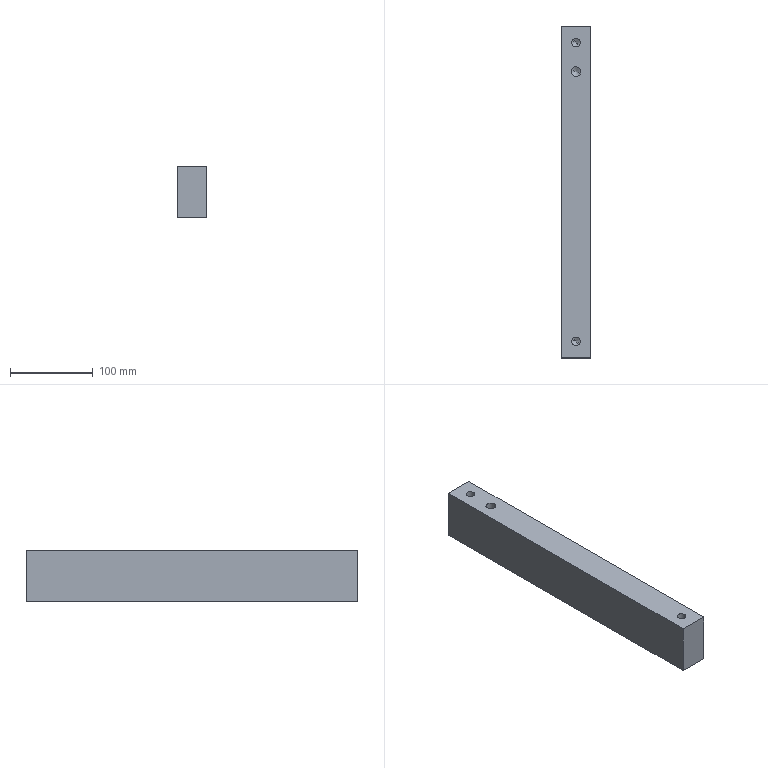Part | CATIA | 1 solid | 38 faces | box 35 x 400 x 61.7 mm | volume 838529 mm3 | cone 16 | cylinder 16 | plane 6 | commonest cylinder face diameters 10.2 x10 12 x6
STEP:
#1=CARTESIAN_POINT('',(-17.5,200.,-275.));
#2=VERTEX_POINT('',#1);
#3=CARTESIAN_POINT('',(-17.5,-200.,-275.));
#4=VERTEX_POINT('',#3);
#5=CARTESIAN_POINT('',(-17.5,0.,-275.));
#6=DIRECTION('',(0.,-1.,0.));
#7=VECTOR('',#6,1.);
#8=LINE('',#5,#7);
#9=EDGE_CURVE('',#2,#4,#8,.T.);
#10=ORIENTED_EDGE('',*,*,#9,.T.);
#11=CARTESIAN_POINT('',(-17.5,-200.,-213.3));
#12=VERTEX_POINT('',#11);
#13=CARTESIAN_POINT('',(-17.5,-200.,-244.15));
#14=DIRECTION('',(0.,0.,-1.));
#15=VECTOR('',#14,1.);
#16=LINE('',#13,#15);
#17=EDGE_CURVE('',#12,#4,#16,.T.);
#18=ORIENTED_EDGE('',*,*,#17,.F.);
#19=CARTESIAN_POINT('',(-17.5,200.,-213.3));
#20=VERTEX_POINT('',#19);
#21=CARTESIAN_POINT('',(-17.5,0.,-213.3));
#22=DIRECTION('',(0.,-1.,0.));
#23=VECTOR('',#22,1.);
#24=LINE('',#21,#23);
#25=EDGE_CURVE('',#20,#12,#24,.T.);
#26=ORIENTED_EDGE('',*,*,#25,.F.);
#27=CARTESIAN_POINT('',(-17.5,200.,-244.15));
#28=DIRECTION('',(0.,0.,-1.));
#29=VECTOR('',#28,1.);
#30=LINE('',#27,#29);
#31=EDGE_CURVE('',#20,#2,#30,.T.);
#32=ORIENTED_EDGE('',*,*,#31,.T.);
#33=EDGE_LOOP('',(#10,#18,#26,#32));
#34=FACE_OUTER_BOUND('',#33,.T.);
#35=CARTESIAN_POINT('',(-17.5,200.,0.));
#36=DIRECTION('',(1.,0.,0.));
#37=DIRECTION('',(0.,-1.,0.));
#38=AXIS2_PLACEMENT_3D('',#35,#36,#37);
#39=PLANE('',#38);
#40=ADVANCED_FACE('',(#34),#39,.F.);
#41=CARTESIAN_POINT('',(17.5,-200.,-275.));
#42=VERTEX_POINT('',#41);
#43=CARTESIAN_POINT('',(0.,-200.,-275.));
#44=DIRECTION('',(-1.,0.,0.));
#45=VECTOR('',#44,1.);
#46=LINE('',#43,#45);
#47=EDGE_CURVE('',#4,#42,#46,.F.);
#48=ORIENTED_EDGE('',*,*,#47,.T.);
#49=CARTESIAN_POINT('',(17.5,-200.,-213.3));
#50=VERTEX_POINT('',#49);
#51=CARTESIAN_POINT('',(17.5,-200.,-244.15));
#52=DIRECTION('',(0.,0.,-1.));
#53=VECTOR('',#52,1.);
#54=LINE('',#51,#53);
#55=EDGE_CURVE('',#50,#42,#54,.T.);
#56=ORIENTED_EDGE('',*,*,#55,.F.);
#57=CARTESIAN_POINT('',(0.,-200.,-213.3));
#58=DIRECTION('',(-1.,0.,0.));
#59=VECTOR('',#58,1.);
#60=LINE('',#57,#59);
#61=EDGE_CURVE('',#12,#50,#60,.F.);
#62=ORIENTED_EDGE('',*,*,#61,.F.);
#63=ORIENTED_EDGE('',*,*,#17,.T.);
#64=EDGE_LOOP('',(#48,#56,#62,#63));
#65=FACE_OUTER_BOUND('',#64,.T.);
#66=CARTESIAN_POINT('',(17.5,-200.,0.));
#67=DIRECTION('',(0.,-1.,0.));
#68=DIRECTION('',(-1.,0.,0.));
#69=AXIS2_PLACEMENT_3D('',#66,#67,#68);
#70=PLANE('',#69);
#71=ADVANCED_FACE('',(#65),#70,.T.);
#72=CARTESIAN_POINT('',(17.5,200.,-275.));
#73=VERTEX_POINT('',#72);
#74=CARTESIAN_POINT('',(17.5,0.,-275.));
#75=DIRECTION('',(0.,1.,0.));
#76=VECTOR('',#75,1.);
#77=LINE('',#74,#76);
#78=EDGE_CURVE('',#42,#73,#77,.T.);
#79=ORIENTED_EDGE('',*,*,#78,.T.);
#80=CARTESIAN_POINT('',(17.5,200.,-213.3));
#81=VERTEX_POINT('',#80);
#82=CARTESIAN_POINT('',(17.5,200.,-244.15));
#83=DIRECTION('',(0.,0.,-1.));
#84=VECTOR('',#83,1.);
#85=LINE('',#82,#84);
#86=EDGE_CURVE('',#81,#73,#85,.T.);
#87=ORIENTED_EDGE('',*,*,#86,.F.);
#88=CARTESIAN_POINT('',(17.5,0.,-213.3));
#89=DIRECTION('',(0.,1.,0.));
#90=VECTOR('',#89,1.);
#91=LINE('',#88,#90);
#92=EDGE_CURVE('',#50,#81,#91,.T.);
#93=ORIENTED_EDGE('',*,*,#92,.F.);
#94=ORIENTED_EDGE('',*,*,#55,.T.);
#95=EDGE_LOOP('',(#79,#87,#93,#94));
#96=FACE_OUTER_BOUND('',#95,.T.);
#97=CARTESIAN_POINT('',(17.5,-200.,0.));
#98=DIRECTION('',(-1.,0.,0.));
#99=DIRECTION('',(0.,1.,0.));
#100=AXIS2_PLACEMENT_3D('',#97,#98,#99);
#101=PLANE('',#100);
#102=ADVANCED_FACE('',(#96),#101,.F.);
#103=CARTESIAN_POINT('',(0.,200.,-275.));
#104=DIRECTION('',(1.,0.,0.));
#105=VECTOR('',#104,1.);
#106=LINE('',#103,#105);
#107=EDGE_CURVE('',#73,#2,#106,.F.);
#108=ORIENTED_EDGE('',*,*,#107,.T.);
#109=ORIENTED_EDGE('',*,*,#31,.F.);
#110=CARTESIAN_POINT('',(0.,200.,-213.3));
#111=DIRECTION('',(1.,0.,0.));
#112=VECTOR('',#111,1.);
#113=LINE('',#110,#112);
#114=EDGE_CURVE('',#81,#20,#113,.F.);
#115=ORIENTED_EDGE('',*,*,#114,.F.);
#116=ORIENTED_EDGE('',*,*,#86,.T.);
#117=EDGE_LOOP('',(#108,#109,#115,#116));
#118=FACE_OUTER_BOUND('',#117,.T.);
#119=CARTESIAN_POINT('',(-17.5,200.,0.));
#120=DIRECTION('',(0.,1.,0.));
#121=DIRECTION('',(1.,0.,0.));
#122=AXIS2_PLACEMENT_3D('',#119,#120,#121);
#123=PLANE('',#122);
#124=ADVANCED_FACE('',(#118),#123,.T.);
#125=ORIENTED_EDGE('',*,*,#107,.F.);
#126=ORIENTED_EDGE('',*,*,#78,.F.);
#127=ORIENTED_EDGE('',*,*,#47,.F.);
#128=ORIENTED_EDGE('',*,*,#9,.F.);
#129=EDGE_LOOP('',(#125,#126,#127,#128));
#130=FACE_OUTER_BOUND('',#129,.T.);
#131=CARTESIAN_POINT('',(4.476,-162.555,-275.));
#132=VERTEX_POINT('',#131);
#133=CARTESIAN_POINT('',(-4.476,-167.445,-275.));
#134=VERTEX_POINT('',#133);
#135=CARTESIAN_POINT('',(0.,-165.,-275.));
#136=DIRECTION('',(0.,0.,1.));
#137=AXIS2_PLACEMENT_3D('',#135,#136,$);
#138=CIRCLE('',#137,5.1);
#139=EDGE_CURVE('',#132,#134,#138,.T.);
#140=ORIENTED_EDGE('',*,*,#139,.T.);
#141=CARTESIAN_POINT('',(0.,-165.,-275.));
#142=DIRECTION('',(0.,0.,1.));
#143=AXIS2_PLACEMENT_3D('',#141,#142,$);
#144=CIRCLE('',#143,5.1);
#145=EDGE_CURVE('',#134,#132,#144,.T.);
#146=ORIENTED_EDGE('',*,*,#145,.T.);
#147=EDGE_LOOP('',(#140,#146));
#148=FACE_BOUND('',#147,.T.);
#149=CARTESIAN_POINT('',(4.476,167.445,-275.));
#150=VERTEX_POINT('',#149);
#151=CARTESIAN_POINT('',(-4.476,162.555,-275.));
#152=VERTEX_POINT('',#151);
#153=CARTESIAN_POINT('',(0.,165.,-275.));
#154=DIRECTION('',(0.,0.,1.));
#155=AXIS2_PLACEMENT_3D('',#153,#154,$);
#156=CIRCLE('',#155,5.1);
#157=EDGE_CURVE('',#150,#152,#156,.T.);
#158=ORIENTED_EDGE('',*,*,#157,.T.);
#159=CARTESIAN_POINT('',(0.,165.,-275.));
#160=DIRECTION('',(0.,0.,1.));
#161=AXIS2_PLACEMENT_3D('',#159,#160,$);
#162=CIRCLE('',#161,5.1);
#163=EDGE_CURVE('',#152,#150,#162,.T.);
#164=ORIENTED_EDGE('',*,*,#163,.T.);
#165=EDGE_LOOP('',(#158,#164));
#166=FACE_BOUND('',#165,.T.);
#167=CARTESIAN_POINT('',(4.476,-7.555,-275.));
#168=VERTEX_POINT('',#167);
#169=CARTESIAN_POINT('',(-4.476,-12.445,-275.));
#170=VERTEX_POINT('',#169);
#171=CARTESIAN_POINT('',(0.,-10.,-275.));
#172=DIRECTION('',(0.,0.,1.));
#173=AXIS2_PLACEMENT_3D('',#171,#172,$);
#174=CIRCLE('',#173,5.1);
#175=EDGE_CURVE('',#168,#170,#174,.T.);
#176=ORIENTED_EDGE('',*,*,#175,.T.);
#177=CARTESIAN_POINT('',(0.,-10.,-275.));
#178=DIRECTION('',(0.,0.,1.));
#179=AXIS2_PLACEMENT_3D('',#177,#178,$);
#180=CIRCLE('',#179,5.1);
#181=EDGE_CURVE('',#170,#168,#180,.T.);
#182=ORIENTED_EDGE('',*,*,#181,.T.);
#183=EDGE_LOOP('',(#176,#182));
#184=FACE_BOUND('',#183,.T.);
#185=CARTESIAN_POINT('',(5.265,-137.123,-275.));
#186=VERTEX_POINT('',#185);
#187=CARTESIAN_POINT('',(-5.265,-142.877,-275.));
#188=VERTEX_POINT('',#187);
#189=CARTESIAN_POINT('',(0.,-140.,-275.));
#190=DIRECTION('',(0.,0.,1.));
#191=AXIS2_PLACEMENT_3D('',#189,#190,$);
#192=CIRCLE('',#191,6.);
#193=EDGE_CURVE('',#186,#188,#192,.T.);
#194=ORIENTED_EDGE('',*,*,#193,.T.);
#195=CARTESIAN_POINT('',(0.,-140.,-275.));
#196=DIRECTION('',(0.,0.,1.));
#197=AXIS2_PLACEMENT_3D('',#195,#196,$);
#198=CIRCLE('',#197,6.);
#199=EDGE_CURVE('',#188,#186,#198,.T.);
#200=ORIENTED_EDGE('',*,*,#199,.T.);
#201=EDGE_LOOP('',(#194,#200));
#202=FACE_BOUND('',#201,.T.);
#203=CARTESIAN_POINT('',(5.265,137.877,-275.));
#204=VERTEX_POINT('',#203);
#205=CARTESIAN_POINT('',(-5.265,132.123,-275.));
#206=VERTEX_POINT('',#205);
#207=CARTESIAN_POINT('',(0.,135.,-275.));
#208=DIRECTION('',(0.,0.,1.));
#209=AXIS2_PLACEMENT_3D('',#207,#208,$);
#210=CIRCLE('',#209,6.);
#211=EDGE_CURVE('',#204,#206,#210,.T.);
#212=ORIENTED_EDGE('',*,*,#211,.T.);
#213=CARTESIAN_POINT('',(0.,135.,-275.));
#214=DIRECTION('',(0.,0.,1.));
#215=AXIS2_PLACEMENT_3D('',#213,#214,$);
#216=CIRCLE('',#215,6.);
#217=EDGE_CURVE('',#206,#204,#216,.T.);
#218=ORIENTED_EDGE('',*,*,#217,.T.);
#219=EDGE_LOOP('',(#212,#218));
#220=FACE_BOUND('',#219,.T.);
#221=CARTESIAN_POINT('',(0.,0.,-275.));
#222=DIRECTION('',(0.,0.,1.));
#223=DIRECTION('',(1.,0.,0.));
#224=AXIS2_PLACEMENT_3D('',#221,#222,#223);
#225=PLANE('',#224);
#226=ADVANCED_FACE('',(#130,#148,#166,#184,#202,#220),#225,.F.);
#227=ORIENTED_EDGE('',*,*,#25,.T.);
#228=ORIENTED_EDGE('',*,*,#61,.T.);
#229=ORIENTED_EDGE('',*,*,#92,.T.);
#230=ORIENTED_EDGE('',*,*,#114,.T.);
#231=EDGE_LOOP('',(#227,#228,#229,#230));
#232=FACE_OUTER_BOUND('',#231,.T.);
#233=CARTESIAN_POINT('',(4.476,-182.445,-213.3));
#234=VERTEX_POINT('',#233);
#235=CARTESIAN_POINT('',(-4.476,-177.555,-213.3));
#236=VERTEX_POINT('',#235);
#237=CARTESIAN_POINT('',(0.,-180.,-213.3));
#238=DIRECTION('',(0.,0.,1.));
#239=AXIS2_PLACEMENT_3D('',#237,#238,$);
#240=CIRCLE('',#239,5.1);
#241=EDGE_CURVE('',#234,#236,#240,.T.);
#242=ORIENTED_EDGE('',*,*,#241,.F.);
#243=CARTESIAN_POINT('',(0.,-180.,-213.3));
#244=DIRECTION('',(0.,0.,1.));
#245=AXIS2_PLACEMENT_3D('',#243,#244,$);
#246=CIRCLE('',#245,5.1);
#247=EDGE_CURVE('',#236,#234,#246,.T.);
#248=ORIENTED_EDGE('',*,*,#247,.F.);
#249=EDGE_LOOP('',(#242,#248));
#250=FACE_BOUND('',#249,.T.);
#251=CARTESIAN_POINT('',(4.476,177.555,-213.3));
#252=VERTEX_POINT('',#251);
#253=CARTESIAN_POINT('',(-4.476,182.445,-213.3));
#254=VERTEX_POINT('',#253);
#255=CARTESIAN_POINT('',(0.,180.,-213.3));
#256=DIRECTION('',(0.,0.,1.));
#257=AXIS2_PLACEMENT_3D('',#255,#256,$);
#258=CIRCLE('',#257,5.1);
#259=EDGE_CURVE('',#252,#254,#258,.T.);
#260=ORIENTED_EDGE('',*,*,#259,.F.);
#261=CARTESIAN_POINT('',(0.,180.,-213.3));
#262=DIRECTION('',(0.,0.,1.));
#263=AXIS2_PLACEMENT_3D('',#261,#262,$);
#264=CIRCLE('',#263,5.1);
#265=EDGE_CURVE('',#254,#252,#264,.T.);
#266=ORIENTED_EDGE('',*,*,#265,.F.);
#267=EDGE_LOOP('',(#260,#266));
#268=FACE_BOUND('',#267,.T.);
#269=CARTESIAN_POINT('',(5.265,142.123,-213.3));
#270=VERTEX_POINT('',#269);
#271=CARTESIAN_POINT('',(-5.265,147.877,-213.3));
#272=VERTEX_POINT('',#271);
#273=CARTESIAN_POINT('',(0.,145.,-213.3));
#274=DIRECTION('',(0.,0.,1.));
#275=AXIS2_PLACEMENT_3D('',#273,#274,$);
#276=CIRCLE('',#275,6.);
#277=EDGE_CURVE('',#270,#272,#276,.T.);
#278=ORIENTED_EDGE('',*,*,#277,.F.);
#279=CARTESIAN_POINT('',(0.,145.,-213.3));
#280=DIRECTION('',(0.,0.,1.));
#281=AXIS2_PLACEMENT_3D('',#279,#280,$);
#282=CIRCLE('',#281,6.);
#283=EDGE_CURVE('',#272,#270,#282,.T.);
#284=ORIENTED_EDGE('',*,*,#283,.F.);
#285=EDGE_LOOP('',(#278,#284));
#286=FACE_BOUND('',#285,.T.);
#287=CARTESIAN_POINT('',(0.,0.,-213.3));
#288=DIRECTION('',(0.,0.,1.));
#289=DIRECTION('',(1.,0.,0.));
#290=AXIS2_PLACEMENT_3D('',#287,#288,#289);
#291=PLANE('',#290);
#292=ADVANCED_FACE('',(#232,#250,#268,#286),#291,.T.);
#293=CARTESIAN_POINT('',(0.,135.,-241.536));
#294=VERTEX_POINT('',#293);
#295=CARTESIAN_POINT('',(-5.265,132.123,-245.));
#296=VERTEX_POINT('',#295);
#297=CARTESIAN_POINT('',(-2.633,133.562,-243.268));
#298=DIRECTION('',(-0.76,-0.4152,-0.5));
#299=VECTOR('',#298,1.);
#300=LINE('',#297,#299);
#301=EDGE_CURVE('',#294,#296,#300,.T.);
#302=ORIENTED_EDGE('',*,*,#301,.T.);
#303=CARTESIAN_POINT('',(5.265,137.877,-245.));
#304=VERTEX_POINT('',#303);
#305=CARTESIAN_POINT('',(0.,135.,-245.));
#306=DIRECTION('',(0.,0.,-1.));
#307=AXIS2_PLACEMENT_3D('',#305,#306,$);
#308=CIRCLE('',#307,6.);
#309=EDGE_CURVE('',#304,#296,#308,.F.);
#310=ORIENTED_EDGE('',*,*,#309,.F.);
#311=CARTESIAN_POINT('',(2.633,136.438,-243.268));
#312=DIRECTION('',(0.76,0.4152,-0.5));
#313=VECTOR('',#312,1.);
#314=LINE('',#311,#313);
#315=EDGE_CURVE('',#294,#304,#314,.T.);
#316=ORIENTED_EDGE('',*,*,#315,.F.);
#317=EDGE_LOOP('',(#302,#310,#316));
#318=FACE_OUTER_BOUND('',#317,.T.);
#319=CARTESIAN_POINT('',(0.,135.,-241.536));
#320=DIRECTION('',(0.,0.,-1.));
#321=DIRECTION('',(0.8776,0.4794,0.));
#322=AXIS2_PLACEMENT_3D('',#319,#320,#321);
#323=CONICAL_SURFACE('',#322,0.,1.047);
#324=ADVANCED_FACE('',(#318),#323,.F.);
#325=ORIENTED_EDGE('',*,*,#315,.T.);
#326=CARTESIAN_POINT('',(0.,135.,-245.));
#327=DIRECTION('',(0.,0.,-1.));
#328=AXIS2_PLACEMENT_3D('',#326,#327,$);
#329=CIRCLE('',#328,6.);
#330=EDGE_CURVE('',#296,#304,#329,.F.);
#331=ORIENTED_EDGE('',*,*,#330,.F.);
#332=ORIENTED_EDGE('',*,*,#301,.F.);
#333=EDGE_LOOP('',(#325,#331,#332));
#334=FACE_OUTER_BOUND('',#333,.T.);
#335=ADVANCED_FACE('',(#334),#323,.F.);
#336=ORIENTED_EDGE('',*,*,#211,.F.);
#337=CARTESIAN_POINT('',(5.265,137.877,-260.2));
#338=DIRECTION('',(0.,0.,1.));
#339=VECTOR('',#338,1.);
#340=LINE('',#337,#339);
#341=EDGE_CURVE('',#304,#204,#340,.F.);
#342=ORIENTED_EDGE('',*,*,#341,.F.);
#343=ORIENTED_EDGE('',*,*,#309,.T.);
#344=CARTESIAN_POINT('',(-5.265,132.123,-260.2));
#345=DIRECTION('',(0.,0.,1.));
#346=VECTOR('',#345,1.);
#347=LINE('',#344,#346);
#348=EDGE_CURVE('',#296,#206,#347,.F.);
#349=ORIENTED_EDGE('',*,*,#348,.T.);
#350=EDGE_LOOP('',(#336,#342,#343,#349));
#351=FACE_OUTER_BOUND('',#350,.T.);
#352=CARTESIAN_POINT('',(0.,135.,-274.9));
#353=DIRECTION('',(0.,0.,1.));
#354=DIRECTION('',(0.8776,0.4794,0.));
#355=AXIS2_PLACEMENT_3D('',#352,#353,#354);
#356=CYLINDRICAL_SURFACE('',#355,6.);
#357=ADVANCED_FACE('',(#351),#356,.F.);
#358=ORIENTED_EDGE('',*,*,#217,.F.);
#359=ORIENTED_EDGE('',*,*,#348,.F.);
#360=ORIENTED_EDGE('',*,*,#330,.T.);
#361=ORIENTED_EDGE('',*,*,#341,.T.);
#362=EDGE_LOOP('',(#358,#359,#360,#361));
#363=FACE_OUTER_BOUND('',#362,.T.);
#364=ADVANCED_FACE('',(#363),#356,.F.);
#365=CARTESIAN_POINT('',(0.,165.,-237.056));
#366=VERTEX_POINT('',#365);
#367=CARTESIAN_POINT('',(-4.476,162.555,-240.));
#368=VERTEX_POINT('',#367);
#369=CARTESIAN_POINT('',(-2.238,163.777,-238.528));
#370=DIRECTION('',(-0.76,-0.4152,-0.5));
#371=VECTOR('',#370,1.);
#372=LINE('',#369,#371);
#373=EDGE_CURVE('',#366,#368,#372,.T.);
#374=ORIENTED_EDGE('',*,*,#373,.T.);
#375=CARTESIAN_POINT('',(4.476,167.445,-240.));
#376=VERTEX_POINT('',#375);
#377=CARTESIAN_POINT('',(0.,165.,-240.));
#378=DIRECTION('',(0.,0.,-1.));
#379=AXIS2_PLACEMENT_3D('',#377,#378,$);
#380=CIRCLE('',#379,5.1);
#381=EDGE_CURVE('',#376,#368,#380,.F.);
#382=ORIENTED_EDGE('',*,*,#381,.F.);
#383=CARTESIAN_POINT('',(2.238,166.223,-238.528));
#384=DIRECTION('',(0.76,0.4152,-0.5));
#385=VECTOR('',#384,1.);
#386=LINE('',#383,#385);
#387=EDGE_CURVE('',#366,#376,#386,.T.);
#388=ORIENTED_EDGE('',*,*,#387,.F.);
#389=EDGE_LOOP('',(#374,#382,#388));
#390=FACE_OUTER_BOUND('',#389,.T.);
#391=CARTESIAN_POINT('',(0.,165.,-237.056));
#392=DIRECTION('',(0.,0.,-1.));
#393=DIRECTION('',(0.8776,0.4794,0.));
#394=AXIS2_PLACEMENT_3D('',#391,#392,#393);
#395=CONICAL_SURFACE('',#394,0.,1.047);
#396=ADVANCED_FACE('',(#390),#395,.F.);
#397=ORIENTED_EDGE('',*,*,#387,.T.);
#398=CARTESIAN_POINT('',(0.,165.,-240.));
#399=DIRECTION('',(0.,0.,-1.));
#400=AXIS2_PLACEMENT_3D('',#398,#399,$);
#401=CIRCLE('',#400,5.1);
#402=EDGE_CURVE('',#368,#376,#401,.F.);
#403=ORIENTED_EDGE('',*,*,#402,.F.);
#404=ORIENTED_EDGE('',*,*,#373,.F.);
#405=EDGE_LOOP('',(#397,#403,#404));
#406=FACE_OUTER_BOUND('',#405,.T.);
#407=ADVANCED_FACE('',(#406),#395,.F.);
#408=ORIENTED_EDGE('',*,*,#157,.F.);
#409=CARTESIAN_POINT('',(4.476,167.445,-257.7));
#410=DIRECTION('',(0.,0.,1.));
#411=VECTOR('',#410,1.);
#412=LINE('',#409,#411);
#413=EDGE_CURVE('',#376,#150,#412,.F.);
#414=ORIENTED_EDGE('',*,*,#413,.F.);
#415=ORIENTED_EDGE('',*,*,#381,.T.);
#416=CARTESIAN_POINT('',(-4.476,162.555,-257.7));
#417=DIRECTION('',(0.,0.,1.));
#418=VECTOR('',#417,1.);
#419=LINE('',#416,#418);
#420=EDGE_CURVE('',#368,#152,#419,.F.);
#421=ORIENTED_EDGE('',*,*,#420,.T.);
#422=EDGE_LOOP('',(#408,#414,#415,#421));
#423=FACE_OUTER_BOUND('',#422,.T.);
#424=CARTESIAN_POINT('',(0.,165.,-274.9));
#425=DIRECTION('',(0.,0.,1.));
#426=DIRECTION('',(0.8776,0.4794,0.));
#427=AXIS2_PLACEMENT_3D('',#424,#425,#426);
#428=CYLINDRICAL_SURFACE('',#427,5.1);
#429=ADVANCED_FACE('',(#423),#428,.F.);
#430=ORIENTED_EDGE('',*,*,#163,.F.);
#431=ORIENTED_EDGE('',*,*,#420,.F.);
#432=ORIENTED_EDGE('',*,*,#402,.T.);
#433=ORIENTED_EDGE('',*,*,#413,.T.);
#434=EDGE_LOOP('',(#430,#431,#432,#433));
#435=FACE_OUTER_BOUND('',#434,.T.);
#436=ADVANCED_FACE('',(#435),#428,.F.);
#437=CARTESIAN_POINT('',(0.,180.,-251.244));
#438=VERTEX_POINT('',#437);
#439=CARTESIAN_POINT('',(-4.476,182.445,-248.3));
#440=VERTEX_POINT('',#439);
#441=CARTESIAN_POINT('',(-2.238,181.223,-249.772));
#442=DIRECTION('',(-0.76,0.4152,0.5));
#443=VECTOR('',#442,1.);
#444=LINE('',#441,#443);
#445=EDGE_CURVE('',#438,#440,#444,.T.);
#446=ORIENTED_EDGE('',*,*,#445,.T.);
#447=CARTESIAN_POINT('',(4.476,177.555,-248.3));
#448=VERTEX_POINT('',#447);
#449=CARTESIAN_POINT('',(0.,180.,-248.3));
#450=DIRECTION('',(0.,0.,1.));
#451=AXIS2_PLACEMENT_3D('',#449,#450,$);
#452=CIRCLE('',#451,5.1);
#453=EDGE_CURVE('',#448,#440,#452,.F.);
#454=ORIENTED_EDGE('',*,*,#453,.F.);
#455=CARTESIAN_POINT('',(2.238,178.777,-249.772));
#456=DIRECTION('',(0.76,-0.4152,0.5));
#457=VECTOR('',#456,1.);
#458=LINE('',#455,#457);
#459=EDGE_CURVE('',#438,#448,#458,.T.);
#460=ORIENTED_EDGE('',*,*,#459,.F.);
#461=EDGE_LOOP('',(#446,#454,#460));
#462=FACE_OUTER_BOUND('',#461,.T.);
#463=CARTESIAN_POINT('',(0.,180.,-251.244));
#464=DIRECTION('',(0.,0.,1.));
#465=DIRECTION('',(0.8776,-0.4794,0.));
#466=AXIS2_PLACEMENT_3D('',#463,#464,#465);
#467=CONICAL_SURFACE('',#466,0.,1.047);
#468=ADVANCED_FACE('',(#462),#467,.F.);
#469=ORIENTED_EDGE('',*,*,#459,.T.);
#470=CARTESIAN_POINT('',(0.,180.,-248.3));
#471=DIRECTION('',(0.,0.,1.));
#472=AXIS2_PLACEMENT_3D('',#470,#471,$);
#473=CIRCLE('',#472,5.1);
#474=EDGE_CURVE('',#440,#448,#473,.F.);
#475=ORIENTED_EDGE('',*,*,#474,.F.);
#476=ORIENTED_EDGE('',*,*,#445,.F.);
#477=EDGE_LOOP('',(#469,#475,#476));
#478=FACE_OUTER_BOUND('',#477,.T.);
#479=ADVANCED_FACE('',(#478),#467,.F.);
#480=ORIENTED_EDGE('',*,*,#265,.T.);
#481=CARTESIAN_POINT('',(4.476,177.555,-230.6));
#482=DIRECTION('',(0.,0.,-1.));
#483=VECTOR('',#482,1.);
#484=LINE('',#481,#483);
#485=EDGE_CURVE('',#448,#252,#484,.F.);
#486=ORIENTED_EDGE('',*,*,#485,.F.);
#487=ORIENTED_EDGE('',*,*,#453,.T.);
#488=CARTESIAN_POINT('',(-4.476,182.445,-230.6));
#489=DIRECTION('',(0.,0.,-1.));
#490=VECTOR('',#489,1.);
#491=LINE('',#488,#490);
#492=EDGE_CURVE('',#440,#254,#491,.F.);
#493=ORIENTED_EDGE('',*,*,#492,.T.);
#494=EDGE_LOOP('',(#480,#486,#487,#493));
#495=FACE_OUTER_BOUND('',#494,.T.);
#496=CARTESIAN_POINT('',(0.,180.,-213.4));
#497=DIRECTION('',(0.,0.,-1.));
#498=DIRECTION('',(0.8776,-0.4794,0.));
#499=AXIS2_PLACEMENT_3D('',#496,#497,#498);
#500=CYLINDRICAL_SURFACE('',#499,5.1);
#501=ADVANCED_FACE('',(#495),#500,.F.);
#502=ORIENTED_EDGE('',*,*,#259,.T.);
#503=ORIENTED_EDGE('',*,*,#492,.F.);
#504=ORIENTED_EDGE('',*,*,#474,.T.);
#505=ORIENTED_EDGE('',*,*,#485,.T.);
#506=EDGE_LOOP('',(#502,#503,#504,#505));
#507=FACE_OUTER_BOUND('',#506,.T.);
#508=ADVANCED_FACE('',(#507),#500,.F.);
#509=CARTESIAN_POINT('',(0.,-10.,-237.056));
#510=VERTEX_POINT('',#509);
#511=CARTESIAN_POINT('',(-4.476,-12.445,-240.));
#512=VERTEX_POINT('',#511);
#513=CARTESIAN_POINT('',(-2.238,-11.223,-238.528));
#514=DIRECTION('',(-0.76,-0.4152,-0.5));
#515=VECTOR('',#514,1.);
#516=LINE('',#513,#515);
#517=EDGE_CURVE('',#510,#512,#516,.T.);
#518=ORIENTED_EDGE('',*,*,#517,.T.);
#519=CARTESIAN_POINT('',(4.476,-7.555,-240.));
#520=VERTEX_POINT('',#519);
#521=CARTESIAN_POINT('',(0.,-10.,-240.));
#522=DIRECTION('',(0.,0.,-1.));
#523=AXIS2_PLACEMENT_3D('',#521,#522,$);
#524=CIRCLE('',#523,5.1);
#525=EDGE_CURVE('',#520,#512,#524,.F.);
#526=ORIENTED_EDGE('',*,*,#525,.F.);
#527=CARTESIAN_POINT('',(2.238,-8.777,-238.528));
#528=DIRECTION('',(0.76,0.4152,-0.5));
#529=VECTOR('',#528,1.);
#530=LINE('',#527,#529);
#531=EDGE_CURVE('',#510,#520,#530,.T.);
#532=ORIENTED_EDGE('',*,*,#531,.F.);
#533=EDGE_LOOP('',(#518,#526,#532));
#534=FACE_OUTER_BOUND('',#533,.T.);
#535=CARTESIAN_POINT('',(0.,-10.,-237.056));
#536=DIRECTION('',(0.,0.,-1.));
#537=DIRECTION('',(0.8776,0.4794,0.));
#538=AXIS2_PLACEMENT_3D('',#535,#536,#537);
#539=CONICAL_SURFACE('',#538,0.,1.047);
#540=ADVANCED_FACE('',(#534),#539,.F.);
#541=ORIENTED_EDGE('',*,*,#531,.T.);
#542=CARTESIAN_POINT('',(0.,-10.,-240.));
#543=DIRECTION('',(0.,0.,-1.));
#544=AXIS2_PLACEMENT_3D('',#542,#543,$);
#545=CIRCLE('',#544,5.1);
#546=EDGE_CURVE('',#512,#520,#545,.F.);
#547=ORIENTED_EDGE('',*,*,#546,.F.);
#548=ORIENTED_EDGE('',*,*,#517,.F.);
#549=EDGE_LOOP('',(#541,#547,#548));
#550=FACE_OUTER_BOUND('',#549,.T.);
#551=ADVANCED_FACE('',(#550),#539,.F.);
#552=ORIENTED_EDGE('',*,*,#175,.F.);
#553=CARTESIAN_POINT('',(4.476,-7.555,-257.7));
#554=DIRECTION('',(0.,0.,1.));
#555=VECTOR('',#554,1.);
#556=LINE('',#553,#555);
#557=EDGE_CURVE('',#520,#168,#556,.F.);
#558=ORIENTED_EDGE('',*,*,#557,.F.);
#559=ORIENTED_EDGE('',*,*,#525,.T.);
#560=CARTESIAN_POINT('',(-4.476,-12.445,-257.7));
#561=DIRECTION('',(0.,0.,1.));
#562=VECTOR('',#561,1.);
#563=LINE('',#560,#562);
#564=EDGE_CURVE('',#512,#170,#563,.F.);
#565=ORIENTED_EDGE('',*,*,#564,.T.);
#566=EDGE_LOOP('',(#552,#558,#559,#565));
#567=FACE_OUTER_BOUND('',#566,.T.);
#568=CARTESIAN_POINT('',(0.,-10.,-274.9));
#569=DIRECTION('',(0.,0.,1.));
#570=DIRECTION('',(0.8776,0.4794,0.));
#571=AXIS2_PLACEMENT_3D('',#568,#569,#570);
#572=CYLINDRICAL_SURFACE('',#571,5.1);
#573=ADVANCED_FACE('',(#567),#572,.F.);
#574=ORIENTED_EDGE('',*,*,#181,.F.);
#575=ORIENTED_EDGE('',*,*,#564,.F.);
#576=ORIENTED_EDGE('',*,*,#546,.T.);
#577=ORIENTED_EDGE('',*,*,#557,.T.);
#578=EDGE_LOOP('',(#574,#575,#576,#577));
#579=FACE_OUTER_BOUND('',#578,.T.);
#580=ADVANCED_FACE('',(#579),#572,.F.);
#581=CARTESIAN_POINT('',(0.,-180.,-251.244));
#582=VERTEX_POINT('',#581);
#583=CARTESIAN_POINT('',(-4.476,-177.555,-248.3));
#584=VERTEX_POINT('',#583);
#585=CARTESIAN_POINT('',(-2.238,-178.777,-249.772));
#586=DIRECTION('',(-0.76,0.4152,0.5));
#587=VECTOR('',#586,1.);
#588=LINE('',#585,#587);
#589=EDGE_CURVE('',#582,#584,#588,.T.);
#590=ORIENTED_EDGE('',*,*,#589,.T.);
#591=CARTESIAN_POINT('',(4.476,-182.445,-248.3));
#592=VERTEX_POINT('',#591);
#593=CARTESIAN_POINT('',(0.,-180.,-248.3));
#594=DIRECTION('',(0.,0.,1.));
#595=AXIS2_PLACEMENT_3D('',#593,#594,$);
#596=CIRCLE('',#595,5.1);
#597=EDGE_CURVE('',#592,#584,#596,.F.);
#598=ORIENTED_EDGE('',*,*,#597,.F.);
#599=CARTESIAN_POINT('',(2.238,-181.223,-249.772));
#600=DIRECTION('',(0.76,-0.4152,0.5));
#601=VECTOR('',#600,1.);
#602=LINE('',#599,#601);
#603=EDGE_CURVE('',#582,#592,#602,.T.);
#604=ORIENTED_EDGE('',*,*,#603,.F.);
#605=EDGE_LOOP('',(#590,#598,#604));
#606=FACE_OUTER_BOUND('',#605,.T.);
#607=CARTESIAN_POINT('',(0.,-180.,-251.244));
#608=DIRECTION('',(0.,0.,1.));
#609=DIRECTION('',(0.8776,-0.4794,0.));
#610=AXIS2_PLACEMENT_3D('',#607,#608,#609);
#611=CONICAL_SURFACE('',#610,0.,1.047);
#612=ADVANCED_FACE('',(#606),#611,.F.);
#613=ORIENTED_EDGE('',*,*,#603,.T.);
#614=CARTESIAN_POINT('',(0.,-180.,-248.3));
#615=DIRECTION('',(0.,0.,1.));
#616=AXIS2_PLACEMENT_3D('',#614,#615,$);
#617=CIRCLE('',#616,5.1);
#618=EDGE_CURVE('',#584,#592,#617,.F.);
#619=ORIENTED_EDGE('',*,*,#618,.F.);
#620=ORIENTED_EDGE('',*,*,#589,.F.);
#621=EDGE_LOOP('',(#613,#619,#620));
#622=FACE_OUTER_BOUND('',#621,.T.);
#623=ADVANCED_FACE('',(#622),#611,.F.);
#624=ORIENTED_EDGE('',*,*,#247,.T.);
#625=CARTESIAN_POINT('',(4.476,-182.445,-230.6));
#626=DIRECTION('',(0.,0.,-1.));
#627=VECTOR('',#626,1.);
#628=LINE('',#625,#627);
#629=EDGE_CURVE('',#592,#234,#628,.F.);
#630=ORIENTED_EDGE('',*,*,#629,.F.);
#631=ORIENTED_EDGE('',*,*,#597,.T.);
#632=CARTESIAN_POINT('',(-4.476,-177.555,-230.6));
#633=DIRECTION('',(0.,0.,-1.));
#634=VECTOR('',#633,1.);
#635=LINE('',#632,#634);
#636=EDGE_CURVE('',#584,#236,#635,.F.);
#637=ORIENTED_EDGE('',*,*,#636,.T.);
#638=EDGE_LOOP('',(#624,#630,#631,#637));
#639=FACE_OUTER_BOUND('',#638,.T.);
#640=CARTESIAN_POINT('',(0.,-180.,-213.4));
#641=DIRECTION('',(0.,0.,-1.));
#642=DIRECTION('',(0.8776,-0.4794,0.));
#643=AXIS2_PLACEMENT_3D('',#640,#641,#642);
#644=CYLINDRICAL_SURFACE('',#643,5.1);
#645=ADVANCED_FACE('',(#639),#644,.F.);
#646=ORIENTED_EDGE('',*,*,#241,.T.);
#647=ORIENTED_EDGE('',*,*,#636,.F.);
#648=ORIENTED_EDGE('',*,*,#618,.T.);
#649=ORIENTED_EDGE('',*,*,#629,.T.);
#650=EDGE_LOOP('',(#646,#647,#648,#649));
#651=FACE_OUTER_BOUND('',#650,.T.);
#652=ADVANCED_FACE('',(#651),#644,.F.);
#653=CARTESIAN_POINT('',(0.,-140.,-241.536));
#654=VERTEX_POINT('',#653);
#655=CARTESIAN_POINT('',(-5.265,-142.877,-245.));
#656=VERTEX_POINT('',#655);
#657=CARTESIAN_POINT('',(-2.633,-141.438,-243.268));
#658=DIRECTION('',(-0.76,-0.4152,-0.5));
#659=VECTOR('',#658,1.);
#660=LINE('',#657,#659);
#661=EDGE_CURVE('',#654,#656,#660,.T.);
#662=ORIENTED_EDGE('',*,*,#661,.T.);
#663=CARTESIAN_POINT('',(5.265,-137.123,-245.));
#664=VERTEX_POINT('',#663);
#665=CARTESIAN_POINT('',(0.,-140.,-245.));
#666=DIRECTION('',(0.,0.,-1.));
#667=AXIS2_PLACEMENT_3D('',#665,#666,$);
#668=CIRCLE('',#667,6.);
#669=EDGE_CURVE('',#664,#656,#668,.F.);
#670=ORIENTED_EDGE('',*,*,#669,.F.);
#671=CARTESIAN_POINT('',(2.633,-138.562,-243.268));
#672=DIRECTION('',(0.76,0.4152,-0.5));
#673=VECTOR('',#672,1.);
#674=LINE('',#671,#673);
#675=EDGE_CURVE('',#654,#664,#674,.T.);
#676=ORIENTED_EDGE('',*,*,#675,.F.);
#677=EDGE_LOOP('',(#662,#670,#676));
#678=FACE_OUTER_BOUND('',#677,.T.);
#679=CARTESIAN_POINT('',(0.,-140.,-241.536));
#680=DIRECTION('',(0.,0.,-1.));
#681=DIRECTION('',(0.8776,0.4794,0.));
#682=AXIS2_PLACEMENT_3D('',#679,#680,#681);
#683=CONICAL_SURFACE('',#682,0.,1.047);
#684=ADVANCED_FACE('',(#678),#683,.F.);
#685=ORIENTED_EDGE('',*,*,#675,.T.);
#686=CARTESIAN_POINT('',(0.,-140.,-245.));
#687=DIRECTION('',(0.,0.,-1.));
#688=AXIS2_PLACEMENT_3D('',#686,#687,$);
#689=CIRCLE('',#688,6.);
#690=EDGE_CURVE('',#656,#664,#689,.F.);
#691=ORIENTED_EDGE('',*,*,#690,.F.);
#692=ORIENTED_EDGE('',*,*,#661,.F.);
#693=EDGE_LOOP('',(#685,#691,#692));
#694=FACE_OUTER_BOUND('',#693,.T.);
#695=ADVANCED_FACE('',(#694),#683,.F.);
#696=ORIENTED_EDGE('',*,*,#193,.F.);
#697=CARTESIAN_POINT('',(5.265,-137.123,-260.2));
#698=DIRECTION('',(0.,0.,1.));
#699=VECTOR('',#698,1.);
#700=LINE('',#697,#699);
#701=EDGE_CURVE('',#664,#186,#700,.F.);
#702=ORIENTED_EDGE('',*,*,#701,.F.);
#703=ORIENTED_EDGE('',*,*,#669,.T.);
#704=CARTESIAN_POINT('',(-5.265,-142.877,-260.2));
#705=DIRECTION('',(0.,0.,1.));
#706=VECTOR('',#705,1.);
#707=LINE('',#704,#706);
#708=EDGE_CURVE('',#656,#188,#707,.F.);
#709=ORIENTED_EDGE('',*,*,#708,.T.);
#710=EDGE_LOOP('',(#696,#702,#703,#709));
#711=FACE_OUTER_BOUND('',#710,.T.);
#712=CARTESIAN_POINT('',(0.,-140.,-274.9));
#713=DIRECTION('',(0.,0.,1.));
#714=DIRECTION('',(0.8776,0.4794,0.));
#715=AXIS2_PLACEMENT_3D('',#712,#713,#714);
#716=CYLINDRICAL_SURFACE('',#715,6.);
#717=ADVANCED_FACE('',(#711),#716,.F.);
#718=ORIENTED_EDGE('',*,*,#199,.F.);
#719=ORIENTED_EDGE('',*,*,#708,.F.);
#720=ORIENTED_EDGE('',*,*,#690,.T.);
#721=ORIENTED_EDGE('',*,*,#701,.T.);
#722=EDGE_LOOP('',(#718,#719,#720,#721));
#723=FACE_OUTER_BOUND('',#722,.T.);
#724=ADVANCED_FACE('',(#723),#716,.F.);
#725=CARTESIAN_POINT('',(0.,145.,-246.764));
#726=VERTEX_POINT('',#725);
#727=CARTESIAN_POINT('',(-5.265,147.877,-243.3));
#728=VERTEX_POINT('',#727);
#729=CARTESIAN_POINT('',(-2.633,146.438,-245.032));
#730=DIRECTION('',(-0.76,0.4152,0.5));
#731=VECTOR('',#730,1.);
#732=LINE('',#729,#731);
#733=EDGE_CURVE('',#726,#728,#732,.T.);
#734=ORIENTED_EDGE('',*,*,#733,.T.);
#735=CARTESIAN_POINT('',(5.265,142.123,-243.3));
#736=VERTEX_POINT('',#735);
#737=CARTESIAN_POINT('',(0.,145.,-243.3));
#738=DIRECTION('',(0.,0.,1.));
#739=AXIS2_PLACEMENT_3D('',#737,#738,$);
#740=CIRCLE('',#739,6.);
#741=EDGE_CURVE('',#736,#728,#740,.F.);
#742=ORIENTED_EDGE('',*,*,#741,.F.);
#743=CARTESIAN_POINT('',(2.633,143.562,-245.032));
#744=DIRECTION('',(0.76,-0.4152,0.5));
#745=VECTOR('',#744,1.);
#746=LINE('',#743,#745);
#747=EDGE_CURVE('',#726,#736,#746,.T.);
#748=ORIENTED_EDGE('',*,*,#747,.F.);
#749=EDGE_LOOP('',(#734,#742,#748));
#750=FACE_OUTER_BOUND('',#749,.T.);
#751=CARTESIAN_POINT('',(0.,145.,-246.764));
#752=DIRECTION('',(0.,0.,1.));
#753=DIRECTION('',(0.8776,-0.4794,0.));
#754=AXIS2_PLACEMENT_3D('',#751,#752,#753);
#755=CONICAL_SURFACE('',#754,0.,1.047);
#756=ADVANCED_FACE('',(#750),#755,.F.);
#757=ORIENTED_EDGE('',*,*,#747,.T.);
#758=CARTESIAN_POINT('',(0.,145.,-243.3));
#759=DIRECTION('',(0.,0.,1.));
#760=AXIS2_PLACEMENT_3D('',#758,#759,$);
#761=CIRCLE('',#760,6.);
#762=EDGE_CURVE('',#728,#736,#761,.F.);
#763=ORIENTED_EDGE('',*,*,#762,.F.);
#764=ORIENTED_EDGE('',*,*,#733,.F.);
#765=EDGE_LOOP('',(#757,#763,#764));
#766=FACE_OUTER_BOUND('',#765,.T.);
#767=ADVANCED_FACE('',(#766),#755,.F.);
#768=ORIENTED_EDGE('',*,*,#283,.T.);
#769=CARTESIAN_POINT('',(5.265,142.123,-228.1));
#770=DIRECTION('',(0.,0.,-1.));
#771=VECTOR('',#770,1.);
#772=LINE('',#769,#771);
#773=EDGE_CURVE('',#736,#270,#772,.F.);
#774=ORIENTED_EDGE('',*,*,#773,.F.);
#775=ORIENTED_EDGE('',*,*,#741,.T.);
#776=CARTESIAN_POINT('',(-5.265,147.877,-228.1));
#777=DIRECTION('',(0.,0.,-1.));
#778=VECTOR('',#777,1.);
#779=LINE('',#776,#778);
#780=EDGE_CURVE('',#728,#272,#779,.F.);
#781=ORIENTED_EDGE('',*,*,#780,.T.);
#782=EDGE_LOOP('',(#768,#774,#775,#781));
#783=FACE_OUTER_BOUND('',#782,.T.);
#784=CARTESIAN_POINT('',(0.,145.,-213.4));
#785=DIRECTION('',(0.,0.,-1.));
#786=DIRECTION('',(0.8776,-0.4794,0.));
#787=AXIS2_PLACEMENT_3D('',#784,#785,#786);
#788=CYLINDRICAL_SURFACE('',#787,6.);
#789=ADVANCED_FACE('',(#783),#788,.F.);
#790=ORIENTED_EDGE('',*,*,#277,.T.);
#791=ORIENTED_EDGE('',*,*,#780,.F.);
#792=ORIENTED_EDGE('',*,*,#762,.T.);
#793=ORIENTED_EDGE('',*,*,#773,.T.);
#794=EDGE_LOOP('',(#790,#791,#792,#793));
#795=FACE_OUTER_BOUND('',#794,.T.);
#796=ADVANCED_FACE('',(#795),#788,.F.);
#797=CARTESIAN_POINT('',(0.,-165.,-237.056));
#798=VERTEX_POINT('',#797);
#799=CARTESIAN_POINT('',(-4.476,-167.445,-240.));
#800=VERTEX_POINT('',#799);
#801=CARTESIAN_POINT('',(-2.238,-166.223,-238.528));
#802=DIRECTION('',(-0.76,-0.4152,-0.5));
#803=VECTOR('',#802,1.);
#804=LINE('',#801,#803);
#805=EDGE_CURVE('',#798,#800,#804,.T.);
#806=ORIENTED_EDGE('',*,*,#805,.T.);
#807=CARTESIAN_POINT('',(4.476,-162.555,-240.));
#808=VERTEX_POINT('',#807);
#809=CARTESIAN_POINT('',(0.,-165.,-240.));
#810=DIRECTION('',(0.,0.,-1.));
#811=AXIS2_PLACEMENT_3D('',#809,#810,$);
#812=CIRCLE('',#811,5.1);
#813=EDGE_CURVE('',#808,#800,#812,.F.);
#814=ORIENTED_EDGE('',*,*,#813,.F.);
#815=CARTESIAN_POINT('',(2.238,-163.777,-238.528));
#816=DIRECTION('',(0.76,0.4152,-0.5));
#817=VECTOR('',#816,1.);
#818=LINE('',#815,#817);
#819=EDGE_CURVE('',#798,#808,#818,.T.);
#820=ORIENTED_EDGE('',*,*,#819,.F.);
#821=EDGE_LOOP('',(#806,#814,#820));
#822=FACE_OUTER_BOUND('',#821,.T.);
#823=CARTESIAN_POINT('',(0.,-165.,-237.056));
#824=DIRECTION('',(0.,0.,-1.));
#825=DIRECTION('',(0.8776,0.4794,0.));
#826=AXIS2_PLACEMENT_3D('',#823,#824,#825);
#827=CONICAL_SURFACE('',#826,0.,1.047);
#828=ADVANCED_FACE('',(#822),#827,.F.);
#829=ORIENTED_EDGE('',*,*,#819,.T.);
#830=CARTESIAN_POINT('',(0.,-165.,-240.));
#831=DIRECTION('',(0.,0.,-1.));
#832=AXIS2_PLACEMENT_3D('',#830,#831,$);
#833=CIRCLE('',#832,5.1);
#834=EDGE_CURVE('',#800,#808,#833,.F.);
#835=ORIENTED_EDGE('',*,*,#834,.F.);
#836=ORIENTED_EDGE('',*,*,#805,.F.);
#837=EDGE_LOOP('',(#829,#835,#836));
#838=FACE_OUTER_BOUND('',#837,.T.);
#839=ADVANCED_FACE('',(#838),#827,.F.);
#840=ORIENTED_EDGE('',*,*,#139,.F.);
#841=CARTESIAN_POINT('',(4.476,-162.555,-257.7));
#842=DIRECTION('',(0.,0.,1.));
#843=VECTOR('',#842,1.);
#844=LINE('',#841,#843);
#845=EDGE_CURVE('',#808,#132,#844,.F.);
#846=ORIENTED_EDGE('',*,*,#845,.F.);
#847=ORIENTED_EDGE('',*,*,#813,.T.);
#848=CARTESIAN_POINT('',(-4.476,-167.445,-257.7));
#849=DIRECTION('',(0.,0.,1.));
#850=VECTOR('',#849,1.);
#851=LINE('',#848,#850);
#852=EDGE_CURVE('',#800,#134,#851,.F.);
#853=ORIENTED_EDGE('',*,*,#852,.T.);
#854=EDGE_LOOP('',(#840,#846,#847,#853));
#855=FACE_OUTER_BOUND('',#854,.T.);
#856=CARTESIAN_POINT('',(0.,-165.,-274.9));
#857=DIRECTION('',(0.,0.,1.));
#858=DIRECTION('',(0.8776,0.4794,0.));
#859=AXIS2_PLACEMENT_3D('',#856,#857,#858);
#860=CYLINDRICAL_SURFACE('',#859,5.1);
#861=ADVANCED_FACE('',(#855),#860,.F.);
#862=ORIENTED_EDGE('',*,*,#145,.F.);
#863=ORIENTED_EDGE('',*,*,#852,.F.);
#864=ORIENTED_EDGE('',*,*,#834,.T.);
#865=ORIENTED_EDGE('',*,*,#845,.T.);
#866=EDGE_LOOP('',(#862,#863,#864,#865));
#867=FACE_OUTER_BOUND('',#866,.T.);
#868=ADVANCED_FACE('',(#867),#860,.F.);
#869=CLOSED_SHELL('',(#40,#71,#102,#124,#226,#292,#324,#335,#357,#364,#396,#407,#429,#436,#468,#479,#501,#508,#540,#551,#573,#580,#612,#623,#645,#652,#684,#695,#717,#724,#756,#767,#789,#796,#828,#839,#861,#868));
#870=MANIFOLD_SOLID_BREP('',#869);
#871=(LENGTH_UNIT()NAMED_UNIT(*)SI_UNIT(.MILLI.,.METRE.));
#872=UNCERTAINTY_MEASURE_WITH_UNIT(LENGTH_MEASURE(0.005),#871,'','');
#873=(NAMED_UNIT(*)PLANE_ANGLE_UNIT()SI_UNIT($,.RADIAN.));
#874=(NAMED_UNIT(*)SI_UNIT($,.STERADIAN.)SOLID_ANGLE_UNIT());
#875=(GEOMETRIC_REPRESENTATION_CONTEXT(3)GLOBAL_UNCERTAINTY_ASSIGNED_CONTEXT((#872))GLOBAL_UNIT_ASSIGNED_CONTEXT((#871,#873,#874))REPRESENTATION_CONTEXT('',''));
#876=ADVANCED_BREP_SHAPE_REPRESENTATION('',(#870),#875);